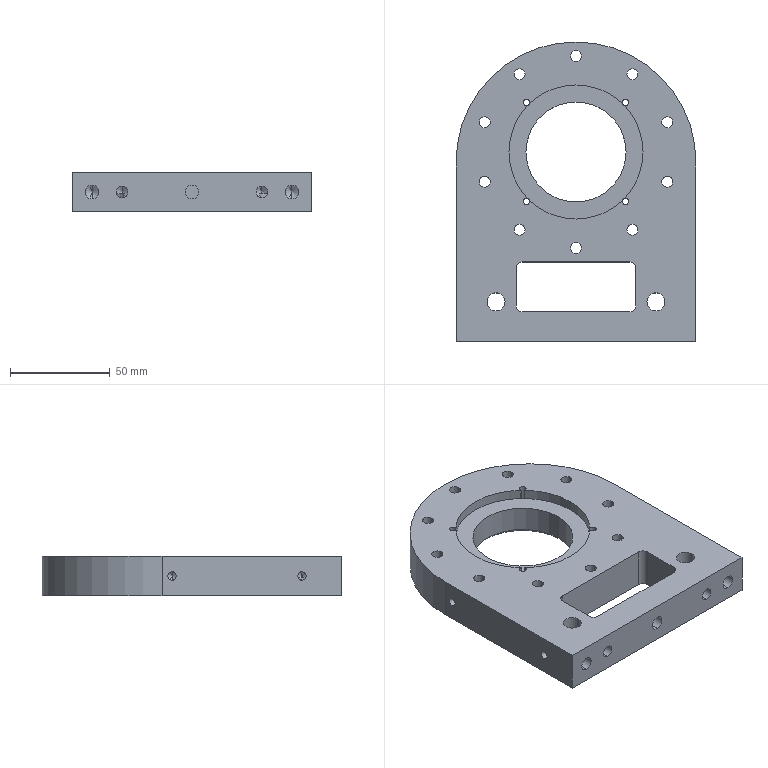Part | SolidWorks | features HoleWzd 6, CirPattern 2, ICE 2, Chamfer 1, Extrusion 1, MirrorPattern 1 | 1 solid | 129 faces | box 120 x 150 x 20 mm | volume 234004 mm3 | cylinder 89 | plane 22 | cone 18 | commonest cylinder face diameters 5.5 x20 10 x20 4.2 x11 3.3 x8 6 x8 6.8 x6